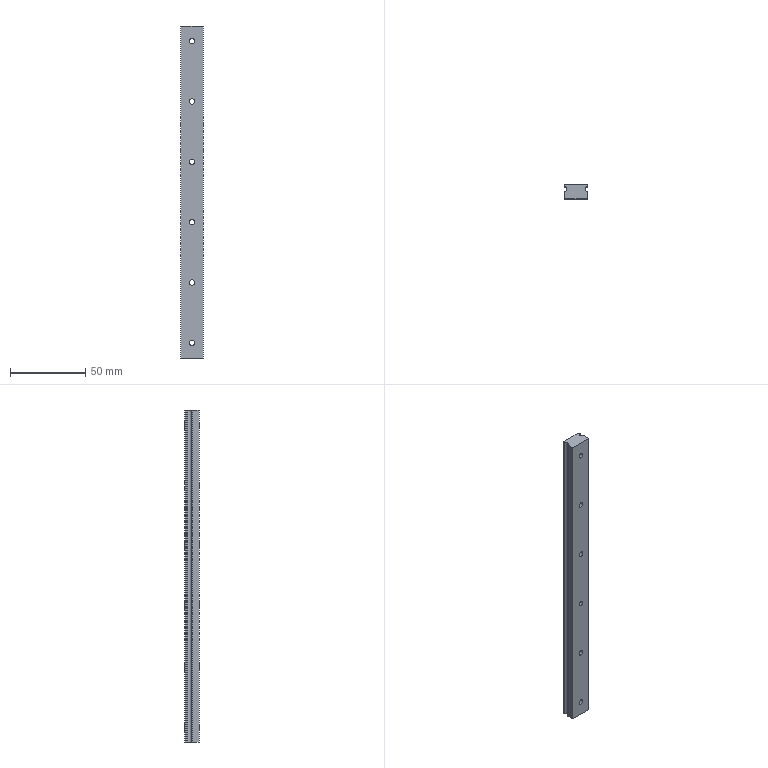Part | STEP file | PN_0015 | 1 solid | 46 faces | box 15 x 9.5 x 220 mm | volume 28688 mm3 | cylinder 32 | plane 14 | commonest cylinder face diameters 3.5 x12 6 x12 1 x6 3 x2